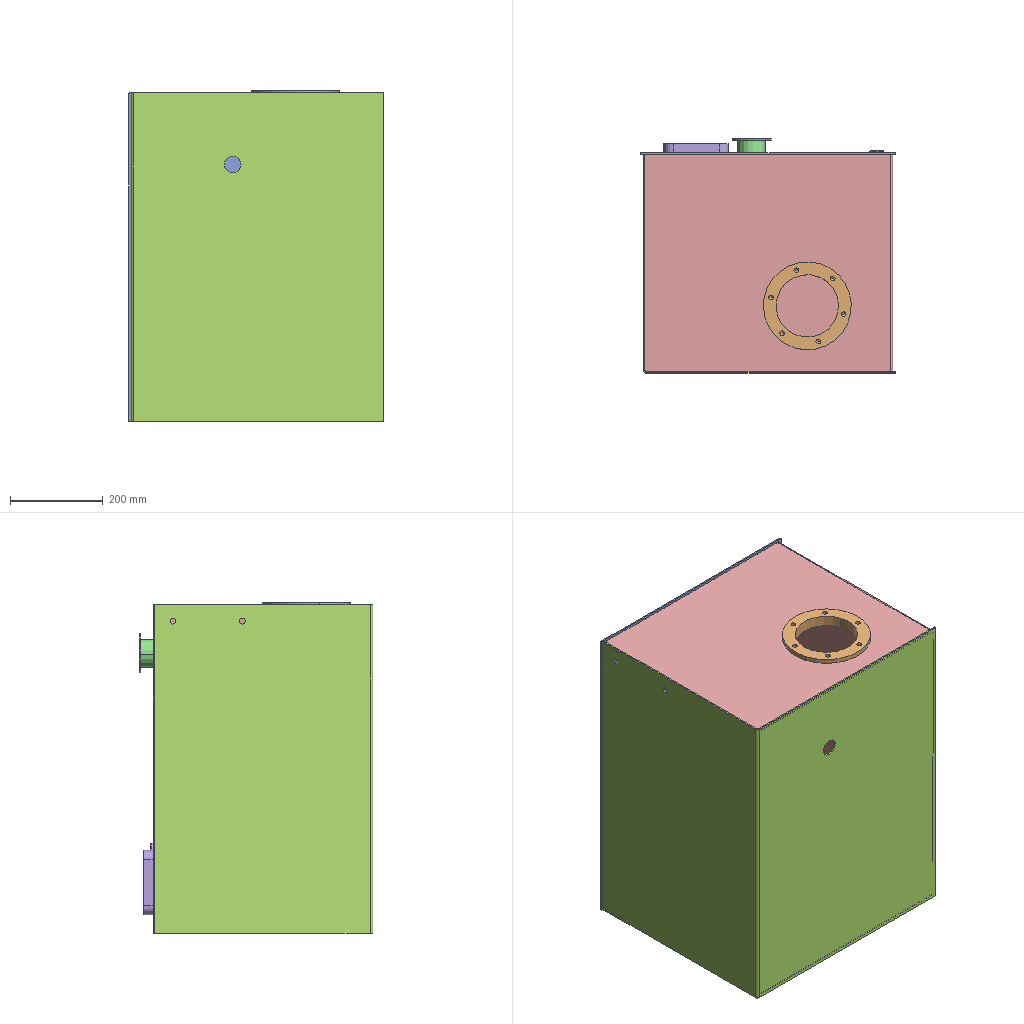Assembly | SolidWorks | 12 different items | 18 placed | box 550 x 505 x 715 mm
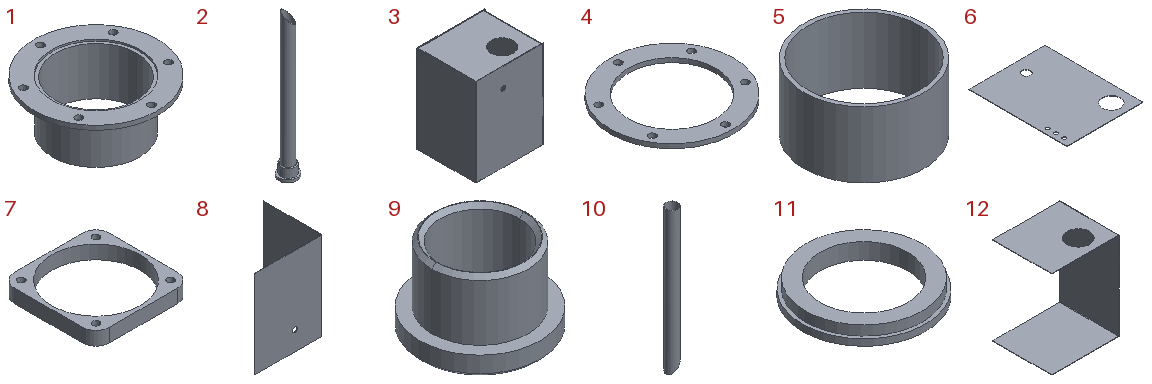Parts list (item | name | quantity | parent item | size | volume | features):
1 | (subassembly) | x1 | - | 85 x 85 x 34 mm | 20100 mm3 | features CompositeCurve 2
2 | (subassembly) | x3 | - | 30 x 30 x 235 mm | 9848 mm3 | features CompositeCurve 2
3 | (subassembly) | x1 | - | 550 x 475 x 710 mm | 5676624 mm3 | -
4 | - | x1 | in 1 | 85 x 85 x 3 mm | 8074 mm3 | features Extrusion 1, ICE 1
5 | - | x1 | in 1 | 60 x 60 x 33 mm | 12026 mm3 | features Extrusion 1
6 | - | x1 | in 3 | 550 x 710 x 3 mm | 1118991 mm3 | features Extrusion 1
7 | - | x1 | - | 140 x 140 x 20 mm | 114105 mm3 | features 3DProfileFeature 1, Extrusion 1, HoleWzd 1
8 | - | x1 | in 3 | 545 x 472 x 710 mm | 2151858 mm3 | features ICE 2, FlatPattern 1, SMBaseFlange 1, SheetMetal 1
9 | - | x3 | in 2 | 30 x 30 x 20 mm | 4047 mm3 | features Chamfer 1, Extrusion 1, ICE 1
10 | - | x3 | in 2 | 18 x 18 x 220 mm | 5800 mm3 | features Extrusion 1, ICE 1
11 | - | x1 | - | 190 x 190 x 25 mm | 301982 mm3 | features 3DProfileFeature 1, Extrusion 1, HoleWzd 1, ICE 1
12 | - | x1 | in 3 | 537.004 x 469 x 699.997 mm | 2405774 mm3 | features ICE 2, FlatPattern 1, SM3dBend 1, SMBaseFlange 1, SheetMetal 1
Mates (type | each side: item.copy, entity, surface, feature):
In the top assembly
Concentric | 6.1 edge | 9.1 edge
Coincident | 6.1 face plane Boss-Extrude1 | 9.1 face plane Boss-Extrude1
Concentric | 6.1 edge | 9.2 edge
Coincident | 6.1 face plane Boss-Extrude1 | 9.2 face plane Boss-Extrude1
Concentric | 6.1 edge | 9.3 edge
Coincident | 6.1 face plane Boss-Extrude1 | 9.3 face plane Boss-Extrude1
Concentric | 12.1 edge | 11.1 edge
Coincident | 12.1 face plane Sketched Bend1 | 11.1 face plane Boss-Extrude1
Coincident | 6.1 face plane Boss-Extrude1 | 7.1 face plane Boss-Extrude1
Concentric | 6.1 edge | 7.1 edge
Perpendicular | 12.1 face plane Base-Flange1 | 7.1 face plane Boss-Extrude1
Concentric | 6.1 edge | 5.1 edge
DistanceDim | 4.1 face plane Boss-Extrude1 | 6.1 face plane Boss-Extrude1
In subassembly 2
Concentric | 9.4 edge | 10.1 edge
DistanceDim | 10.1 face plane Boss-Extrude1 | 9.4 face plane Boss-Extrude1
In subassembly 1
Concentric | 5.2 edge | 4.2 edge
DistanceDim | 4.2 face plane Boss-Extrude1 | 5.2 face plane Boss-Extrude1
In subassembly 3
Coincident | 12.2 face plane Base-Flange1 | 6.2 face plane Boss-Extrude1
DistanceDim | 6.2 face plane Boss-Extrude1 | 12.2 face plane Sketched Bend1
Coincident | 12.2 face plane Base-Flange1 | 8.1 face plane Base-Flange1
DistanceDim | 12.2 face plane Sketched Bend1 | 8.1 face plane Base-Flange1
Coincident | 6.2 face plane Boss-Extrude1 | 8.1 face plane Base-Flange1